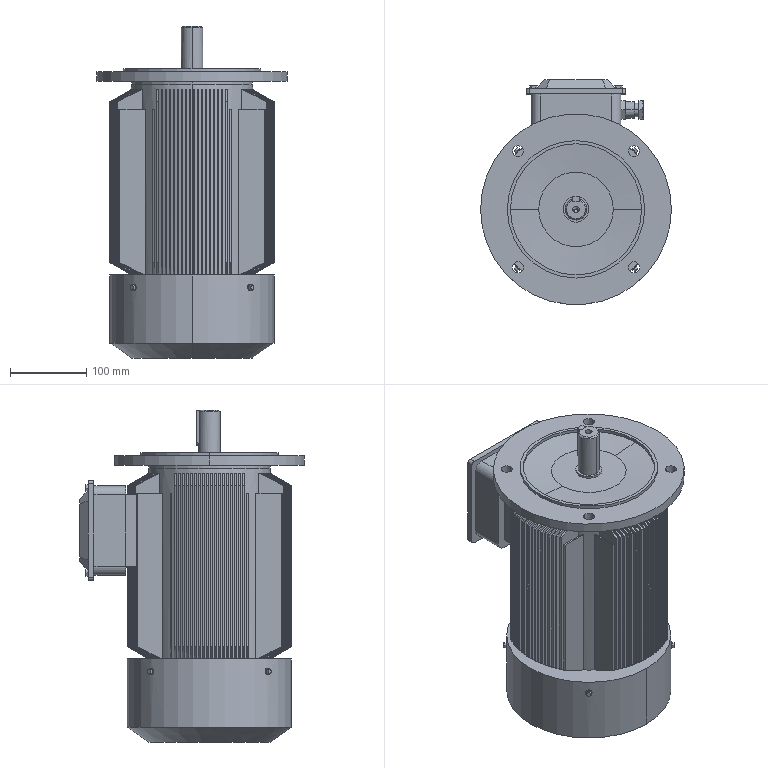Part | STEP file | Produce dryer YE3-100L-4-B5_YE4-100L-2 | 2 solids | 688 faces | box 250 x 295 x 435 mm | volume 12374001 mm3 | plane 299 | cone 247 | cylinder 138 | torus 4 | commonest cylinder face diameters 215 x82 8.6 x8 14.5 x8 7.83 x4 12 x4 18 x4